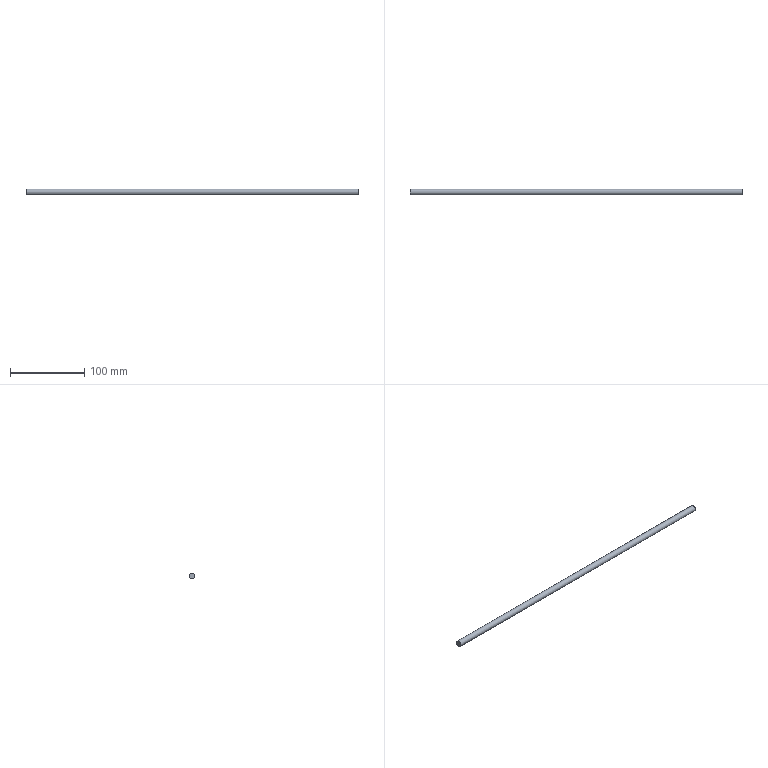Part | NX | features solid 2 | 1 solid | 3 faces | box 447.408 x 8 x 8 mm | volume 22489 mm3 | plane 2 | cylinder 1 | commonest cylinder face diameters 8 x1
STEP:
#1=CARTESIAN_POINT('',(200.,15.,76.5));
#2=VERTEX_POINT('',#1);
#3=CARTESIAN_POINT('',(200.,15.,80.5));
#4=DIRECTION('',(1.,0.,0.));
#5=DIRECTION('',(0.,0.,-1.));
#6=AXIS2_PLACEMENT_3D('',#3,#4,#5);
#7=CIRCLE('',#6,4.);
#8=EDGE_CURVE('',#2,#2,#7,.F.);
#9=ORIENTED_EDGE('',*,*,#8,.F.);
#10=EDGE_LOOP('',(#9));
#11=FACE_BOUND('',#10,.T.);
#12=CARTESIAN_POINT('',(200.,30.064,80.5));
#13=DIRECTION('',(1.,0.,0.));
#14=DIRECTION('',(0.,0.,-1.));
#15=AXIS2_PLACEMENT_3D('',#12,#13,#14);
#16=PLANE('',#15);
#17=ADVANCED_FACE('',(#11),#16,.T.);
#18=CARTESIAN_POINT('',(-247.408,15.,84.5));
#19=VERTEX_POINT('',#18);
#20=CARTESIAN_POINT('',(-247.408,15.,80.5));
#21=DIRECTION('',(-1.,0.,0.));
#22=DIRECTION('',(0.,0.,1.));
#23=AXIS2_PLACEMENT_3D('',#20,#21,#22);
#24=CIRCLE('',#23,4.);
#25=EDGE_CURVE('',#19,#19,#24,.F.);
#26=ORIENTED_EDGE('',*,*,#25,.F.);
#27=EDGE_LOOP('',(#26));
#28=FACE_BOUND('',#27,.T.);
#29=CARTESIAN_POINT('',(-247.408,15.,80.5));
#30=DIRECTION('',(-1.,0.,0.));
#31=DIRECTION('',(0.,0.,1.));
#32=AXIS2_PLACEMENT_3D('',#29,#30,#31);
#33=PLANE('',#32);
#34=ADVANCED_FACE('',(#28),#33,.T.);
#35=ORIENTED_EDGE('',*,*,#8,.T.);
#36=EDGE_LOOP('',(#35));
#37=FACE_BOUND('',#36,.T.);
#38=ORIENTED_EDGE('',*,*,#25,.T.);
#39=EDGE_LOOP('',(#38));
#40=FACE_BOUND('',#39,.T.);
#41=CARTESIAN_POINT('',(-27.408,15.,80.5));
#42=DIRECTION('',(1.,0.,0.));
#43=DIRECTION('',(0.,0.,-1.));
#44=AXIS2_PLACEMENT_3D('',#41,#42,#43);
#45=CYLINDRICAL_SURFACE('',#44,4.);
#46=ADVANCED_FACE('',(#37,#40),#45,.T.);
#47=CLOSED_SHELL('',(#17,#34,#46));
#48=MANIFOLD_SOLID_BREP('',#47);
#49=(LENGTH_UNIT()NAMED_UNIT(*)SI_UNIT(.MILLI.,.METRE.));
#50=UNCERTAINTY_MEASURE_WITH_UNIT(LENGTH_MEASURE(0.00001),#49,'','');
#51=(NAMED_UNIT(*)PLANE_ANGLE_UNIT()SI_UNIT($,.RADIAN.));
#52=(NAMED_UNIT(*)SI_UNIT($,.STERADIAN.)SOLID_ANGLE_UNIT());
#53=(GEOMETRIC_REPRESENTATION_CONTEXT(3)GLOBAL_UNCERTAINTY_ASSIGNED_CONTEXT((#50))GLOBAL_UNIT_ASSIGNED_CONTEXT((#49,#51,#52))REPRESENTATION_CONTEXT('',''));
#54=ADVANCED_BREP_SHAPE_REPRESENTATION('',(#48),#53);